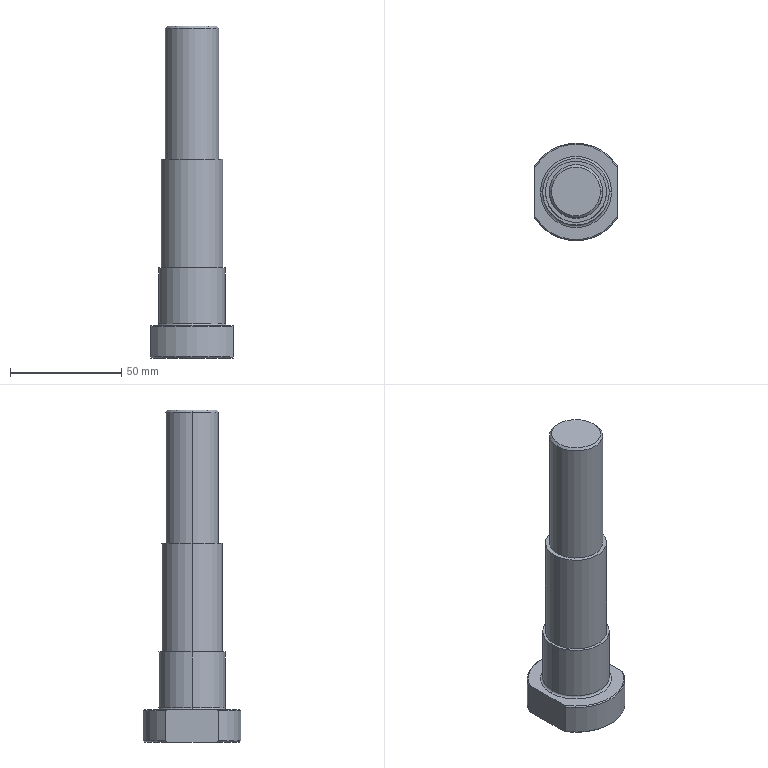Part | STEP file | LM-05-1234 | 1 solid | 23 faces | box 37 x 44 x 149.3 mm | volume 94878 mm3 | cylinder 8 | plane 7 | cone 6 | torus 2 | commonest cylinder face diameters 24 x2 27.5 x2 30 x2 44 x2